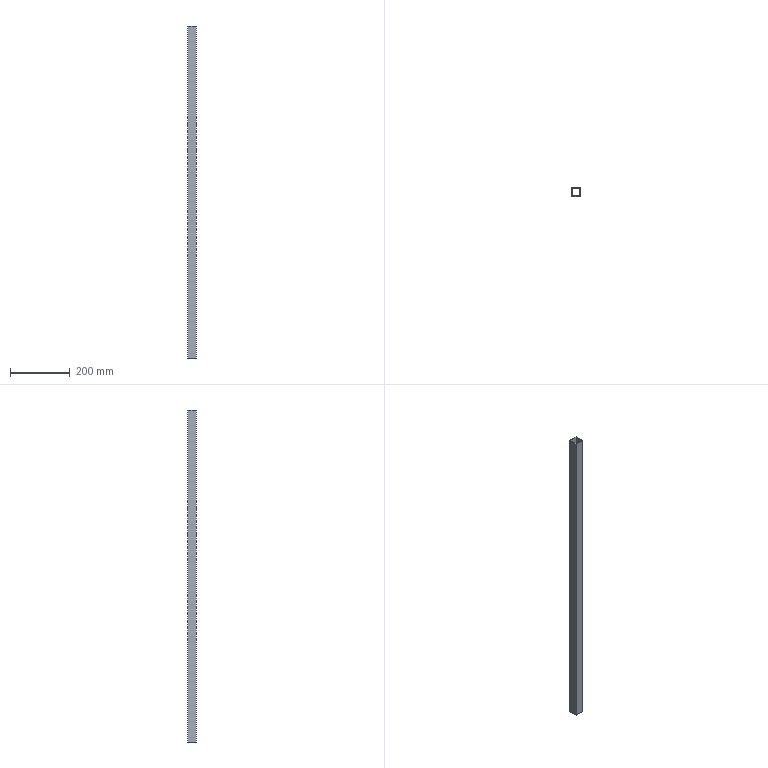Part | SolidWorks | features Extrusion 1 | 1 solid | 10 faces | box 30 x 30 x 1112 mm | volume 249088 mm3 | plane 10
STEP:
#1=CARTESIAN_POINT('',(-15.,15.,556.));
#2=VERTEX_POINT('',#1);
#3=CARTESIAN_POINT('',(-15.,-15.,556.));
#4=VERTEX_POINT('',#3);
#5=CARTESIAN_POINT('',(-15.,-15.,556.));
#6=DIRECTION('',(0.,-1.,0.));
#7=VECTOR('',#6,1000.);
#8=LINE('',#5,#7);
#9=EDGE_CURVE('',#2,#4,#8,.T.);
#10=ORIENTED_EDGE('',*,*,#9,.T.);
#11=CARTESIAN_POINT('',(15.,-15.,556.));
#12=VERTEX_POINT('',#11);
#13=CARTESIAN_POINT('',(15.,-15.,556.));
#14=DIRECTION('',(1.,0.,0.));
#15=VECTOR('',#14,1000.);
#16=LINE('',#13,#15);
#17=EDGE_CURVE('',#4,#12,#16,.T.);
#18=ORIENTED_EDGE('',*,*,#17,.T.);
#19=CARTESIAN_POINT('',(15.,15.,556.));
#20=VERTEX_POINT('',#19);
#21=CARTESIAN_POINT('',(15.,-15.,556.));
#22=DIRECTION('',(0.,1.,0.));
#23=VECTOR('',#22,1000.);
#24=LINE('',#21,#23);
#25=EDGE_CURVE('',#12,#20,#24,.T.);
#26=ORIENTED_EDGE('',*,*,#25,.T.);
#27=CARTESIAN_POINT('',(15.,15.,556.));
#28=DIRECTION('',(-1.,0.,0.));
#29=VECTOR('',#28,1000.);
#30=LINE('',#27,#29);
#31=EDGE_CURVE('',#20,#2,#30,.T.);
#32=ORIENTED_EDGE('',*,*,#31,.T.);
#33=EDGE_LOOP('',(#10,#18,#26,#32));
#34=FACE_OUTER_BOUND('',#33,.T.);
#35=CARTESIAN_POINT('',(13.,13.,556.));
#36=VERTEX_POINT('',#35);
#37=CARTESIAN_POINT('',(-13.,13.,556.));
#38=VERTEX_POINT('',#37);
#39=CARTESIAN_POINT('',(13.,13.,556.));
#40=DIRECTION('',(-1.,0.,0.));
#41=VECTOR('',#40,1000.);
#42=LINE('',#39,#41);
#43=EDGE_CURVE('',#36,#38,#42,.T.);
#44=ORIENTED_EDGE('',*,*,#43,.F.);
#45=CARTESIAN_POINT('',(13.,-13.,556.));
#46=VERTEX_POINT('',#45);
#47=CARTESIAN_POINT('',(13.,-13.,556.));
#48=DIRECTION('',(0.,1.,0.));
#49=VECTOR('',#48,1000.);
#50=LINE('',#47,#49);
#51=EDGE_CURVE('',#46,#36,#50,.T.);
#52=ORIENTED_EDGE('',*,*,#51,.F.);
#53=CARTESIAN_POINT('',(-13.,-13.,556.));
#54=VERTEX_POINT('',#53);
#55=CARTESIAN_POINT('',(13.,-13.,556.));
#56=DIRECTION('',(1.,0.,0.));
#57=VECTOR('',#56,1000.);
#58=LINE('',#55,#57);
#59=EDGE_CURVE('',#54,#46,#58,.T.);
#60=ORIENTED_EDGE('',*,*,#59,.F.);
#61=CARTESIAN_POINT('',(-13.,-13.,556.));
#62=DIRECTION('',(0.,-1.,0.));
#63=VECTOR('',#62,1000.);
#64=LINE('',#61,#63);
#65=EDGE_CURVE('',#38,#54,#64,.T.);
#66=ORIENTED_EDGE('',*,*,#65,.F.);
#67=EDGE_LOOP('',(#44,#52,#60,#66));
#68=FACE_BOUND('',#67,.T.);
#69=CARTESIAN_POINT('',(0.,0.,556.));
#70=DIRECTION('',(0.,0.,1.));
#71=DIRECTION('',(1.,0.,0.));
#72=AXIS2_PLACEMENT_3D('',#69,#70,#71);
#73=PLANE('',#72);
#74=ADVANCED_FACE('',(#34,#68),#73,.T.);
#75=CARTESIAN_POINT('',(-15.,15.,-556.));
#76=VERTEX_POINT('',#75);
#77=CARTESIAN_POINT('',(-15.,-15.,-556.));
#78=VERTEX_POINT('',#77);
#79=CARTESIAN_POINT('',(-15.,-15.,-556.));
#80=DIRECTION('',(0.,-1.,0.));
#81=VECTOR('',#80,1000.);
#82=LINE('',#79,#81);
#83=EDGE_CURVE('',#76,#78,#82,.T.);
#84=ORIENTED_EDGE('',*,*,#83,.F.);
#85=CARTESIAN_POINT('',(15.,15.,-556.));
#86=VERTEX_POINT('',#85);
#87=CARTESIAN_POINT('',(15.,15.,-556.));
#88=DIRECTION('',(-1.,0.,0.));
#89=VECTOR('',#88,1000.);
#90=LINE('',#87,#89);
#91=EDGE_CURVE('',#86,#76,#90,.T.);
#92=ORIENTED_EDGE('',*,*,#91,.F.);
#93=CARTESIAN_POINT('',(15.,-15.,-556.));
#94=VERTEX_POINT('',#93);
#95=CARTESIAN_POINT('',(15.,-15.,-556.));
#96=DIRECTION('',(0.,1.,0.));
#97=VECTOR('',#96,1000.);
#98=LINE('',#95,#97);
#99=EDGE_CURVE('',#94,#86,#98,.T.);
#100=ORIENTED_EDGE('',*,*,#99,.F.);
#101=CARTESIAN_POINT('',(15.,-15.,-556.));
#102=DIRECTION('',(1.,0.,0.));
#103=VECTOR('',#102,1000.);
#104=LINE('',#101,#103);
#105=EDGE_CURVE('',#78,#94,#104,.T.);
#106=ORIENTED_EDGE('',*,*,#105,.F.);
#107=EDGE_LOOP('',(#84,#92,#100,#106));
#108=FACE_OUTER_BOUND('',#107,.T.);
#109=CARTESIAN_POINT('',(13.,-13.,-556.));
#110=VERTEX_POINT('',#109);
#111=CARTESIAN_POINT('',(13.,13.,-556.));
#112=VERTEX_POINT('',#111);
#113=CARTESIAN_POINT('',(13.,-13.,-556.));
#114=DIRECTION('',(0.,1.,0.));
#115=VECTOR('',#114,1000.);
#116=LINE('',#113,#115);
#117=EDGE_CURVE('',#110,#112,#116,.T.);
#118=ORIENTED_EDGE('',*,*,#117,.T.);
#119=CARTESIAN_POINT('',(-13.,13.,-556.));
#120=VERTEX_POINT('',#119);
#121=CARTESIAN_POINT('',(13.,13.,-556.));
#122=DIRECTION('',(-1.,0.,0.));
#123=VECTOR('',#122,1000.);
#124=LINE('',#121,#123);
#125=EDGE_CURVE('',#112,#120,#124,.T.);
#126=ORIENTED_EDGE('',*,*,#125,.T.);
#127=CARTESIAN_POINT('',(-13.,-13.,-556.));
#128=VERTEX_POINT('',#127);
#129=CARTESIAN_POINT('',(-13.,-13.,-556.));
#130=DIRECTION('',(0.,-1.,0.));
#131=VECTOR('',#130,1000.);
#132=LINE('',#129,#131);
#133=EDGE_CURVE('',#120,#128,#132,.T.);
#134=ORIENTED_EDGE('',*,*,#133,.T.);
#135=CARTESIAN_POINT('',(13.,-13.,-556.));
#136=DIRECTION('',(1.,0.,0.));
#137=VECTOR('',#136,1000.);
#138=LINE('',#135,#137);
#139=EDGE_CURVE('',#128,#110,#138,.T.);
#140=ORIENTED_EDGE('',*,*,#139,.T.);
#141=EDGE_LOOP('',(#118,#126,#134,#140));
#142=FACE_BOUND('',#141,.T.);
#143=CARTESIAN_POINT('',(0.,0.,-556.));
#144=DIRECTION('',(0.,0.,1.));
#145=DIRECTION('',(1.,0.,0.));
#146=AXIS2_PLACEMENT_3D('',#143,#144,#145);
#147=PLANE('',#146);
#148=ADVANCED_FACE('',(#108,#142),#147,.F.);
#149=ORIENTED_EDGE('',*,*,#83,.T.);
#150=CARTESIAN_POINT('',(-15.,-15.,556.));
#151=DIRECTION('',(0.,0.,-1.));
#152=VECTOR('',#151,1000.);
#153=LINE('',#150,#152);
#154=EDGE_CURVE('',#4,#78,#153,.T.);
#155=ORIENTED_EDGE('',*,*,#154,.F.);
#156=ORIENTED_EDGE('',*,*,#9,.F.);
#157=CARTESIAN_POINT('',(-15.,15.,556.));
#158=DIRECTION('',(0.,0.,-1.));
#159=VECTOR('',#158,1000.);
#160=LINE('',#157,#159);
#161=EDGE_CURVE('',#2,#76,#160,.T.);
#162=ORIENTED_EDGE('',*,*,#161,.T.);
#163=EDGE_LOOP('',(#149,#155,#156,#162));
#164=FACE_OUTER_BOUND('',#163,.T.);
#165=CARTESIAN_POINT('',(-15.,-15.,556.));
#166=DIRECTION('',(1.,0.,0.));
#167=DIRECTION('',(0.,1.,0.));
#168=AXIS2_PLACEMENT_3D('',#165,#166,#167);
#169=PLANE('',#168);
#170=ADVANCED_FACE('',(#164),#169,.F.);
#171=ORIENTED_EDGE('',*,*,#105,.T.);
#172=CARTESIAN_POINT('',(15.,-15.,556.));
#173=DIRECTION('',(0.,0.,-1.));
#174=VECTOR('',#173,1000.);
#175=LINE('',#172,#174);
#176=EDGE_CURVE('',#12,#94,#175,.T.);
#177=ORIENTED_EDGE('',*,*,#176,.F.);
#178=ORIENTED_EDGE('',*,*,#17,.F.);
#179=ORIENTED_EDGE('',*,*,#154,.T.);
#180=EDGE_LOOP('',(#171,#177,#178,#179));
#181=FACE_OUTER_BOUND('',#180,.T.);
#182=CARTESIAN_POINT('',(15.,-15.,556.));
#183=DIRECTION('',(0.,1.,0.));
#184=DIRECTION('',(-1.,0.,0.));
#185=AXIS2_PLACEMENT_3D('',#182,#183,#184);
#186=PLANE('',#185);
#187=ADVANCED_FACE('',(#181),#186,.F.);
#188=ORIENTED_EDGE('',*,*,#99,.T.);
#189=CARTESIAN_POINT('',(15.,15.,556.));
#190=DIRECTION('',(0.,0.,-1.));
#191=VECTOR('',#190,1000.);
#192=LINE('',#189,#191);
#193=EDGE_CURVE('',#20,#86,#192,.T.);
#194=ORIENTED_EDGE('',*,*,#193,.F.);
#195=ORIENTED_EDGE('',*,*,#25,.F.);
#196=ORIENTED_EDGE('',*,*,#176,.T.);
#197=EDGE_LOOP('',(#188,#194,#195,#196));
#198=FACE_OUTER_BOUND('',#197,.T.);
#199=CARTESIAN_POINT('',(15.,-15.,556.));
#200=DIRECTION('',(-1.,0.,0.));
#201=DIRECTION('',(0.,0.,1.));
#202=AXIS2_PLACEMENT_3D('',#199,#200,#201);
#203=PLANE('',#202);
#204=ADVANCED_FACE('',(#198),#203,.F.);
#205=ORIENTED_EDGE('',*,*,#91,.T.);
#206=ORIENTED_EDGE('',*,*,#161,.F.);
#207=ORIENTED_EDGE('',*,*,#31,.F.);
#208=ORIENTED_EDGE('',*,*,#193,.T.);
#209=EDGE_LOOP('',(#205,#206,#207,#208));
#210=FACE_OUTER_BOUND('',#209,.T.);
#211=CARTESIAN_POINT('',(15.,15.,556.));
#212=DIRECTION('',(0.,-1.,0.));
#213=DIRECTION('',(0.,0.,-1.));
#214=AXIS2_PLACEMENT_3D('',#211,#212,#213);
#215=PLANE('',#214);
#216=ADVANCED_FACE('',(#210),#215,.F.);
#217=ORIENTED_EDGE('',*,*,#117,.F.);
#218=CARTESIAN_POINT('',(13.,-13.,556.));
#219=DIRECTION('',(0.,0.,-1.));
#220=VECTOR('',#219,1000.);
#221=LINE('',#218,#220);
#222=EDGE_CURVE('',#46,#110,#221,.T.);
#223=ORIENTED_EDGE('',*,*,#222,.F.);
#224=ORIENTED_EDGE('',*,*,#51,.T.);
#225=CARTESIAN_POINT('',(13.,13.,556.));
#226=DIRECTION('',(0.,0.,-1.));
#227=VECTOR('',#226,1000.);
#228=LINE('',#225,#227);
#229=EDGE_CURVE('',#36,#112,#228,.T.);
#230=ORIENTED_EDGE('',*,*,#229,.T.);
#231=EDGE_LOOP('',(#217,#223,#224,#230));
#232=FACE_OUTER_BOUND('',#231,.T.);
#233=CARTESIAN_POINT('',(13.,-13.,556.));
#234=DIRECTION('',(-1.,0.,0.));
#235=DIRECTION('',(0.,0.,1.));
#236=AXIS2_PLACEMENT_3D('',#233,#234,#235);
#237=PLANE('',#236);
#238=ADVANCED_FACE('',(#232),#237,.T.);
#239=ORIENTED_EDGE('',*,*,#125,.F.);
#240=ORIENTED_EDGE('',*,*,#229,.F.);
#241=ORIENTED_EDGE('',*,*,#43,.T.);
#242=CARTESIAN_POINT('',(-13.,13.,556.));
#243=DIRECTION('',(0.,0.,-1.));
#244=VECTOR('',#243,1000.);
#245=LINE('',#242,#244);
#246=EDGE_CURVE('',#38,#120,#245,.T.);
#247=ORIENTED_EDGE('',*,*,#246,.T.);
#248=EDGE_LOOP('',(#239,#240,#241,#247));
#249=FACE_OUTER_BOUND('',#248,.T.);
#250=CARTESIAN_POINT('',(13.,13.,556.));
#251=DIRECTION('',(0.,-1.,0.));
#252=DIRECTION('',(0.,0.,-1.));
#253=AXIS2_PLACEMENT_3D('',#250,#251,#252);
#254=PLANE('',#253);
#255=ADVANCED_FACE('',(#249),#254,.T.);
#256=ORIENTED_EDGE('',*,*,#133,.F.);
#257=ORIENTED_EDGE('',*,*,#246,.F.);
#258=ORIENTED_EDGE('',*,*,#65,.T.);
#259=CARTESIAN_POINT('',(-13.,-13.,556.));
#260=DIRECTION('',(0.,0.,-1.));
#261=VECTOR('',#260,1000.);
#262=LINE('',#259,#261);
#263=EDGE_CURVE('',#54,#128,#262,.T.);
#264=ORIENTED_EDGE('',*,*,#263,.T.);
#265=EDGE_LOOP('',(#256,#257,#258,#264));
#266=FACE_OUTER_BOUND('',#265,.T.);
#267=CARTESIAN_POINT('',(-13.,-13.,556.));
#268=DIRECTION('',(1.,0.,0.));
#269=DIRECTION('',(0.,0.,-1.));
#270=AXIS2_PLACEMENT_3D('',#267,#268,#269);
#271=PLANE('',#270);
#272=ADVANCED_FACE('',(#266),#271,.T.);
#273=ORIENTED_EDGE('',*,*,#139,.F.);
#274=ORIENTED_EDGE('',*,*,#263,.F.);
#275=ORIENTED_EDGE('',*,*,#59,.T.);
#276=ORIENTED_EDGE('',*,*,#222,.T.);
#277=EDGE_LOOP('',(#273,#274,#275,#276));
#278=FACE_OUTER_BOUND('',#277,.T.);
#279=CARTESIAN_POINT('',(13.,-13.,556.));
#280=DIRECTION('',(0.,1.,0.));
#281=DIRECTION('',(0.,0.,1.));
#282=AXIS2_PLACEMENT_3D('',#279,#280,#281);
#283=PLANE('',#282);
#284=ADVANCED_FACE('',(#278),#283,.T.);
#285=CLOSED_SHELL('',(#74,#148,#170,#187,#204,#216,#238,#255,#272,#284));
#286=MANIFOLD_SOLID_BREP('',#285);
#287=CARTESIAN_POINT('',(0.,0.,0.));
#288=DIRECTION('',(0.,0.,1.));
#289=DIRECTION('',(1.,0.,0.));
#290=AXIS2_PLACEMENT_3D('',#287,#288,#289);
#291=(LENGTH_UNIT()NAMED_UNIT(*)SI_UNIT(.MILLI.,.METRE.));
#292=UNCERTAINTY_MEASURE_WITH_UNIT(LENGTH_MEASURE(0.00001),#291,'','');
#293=(NAMED_UNIT(*)PLANE_ANGLE_UNIT()SI_UNIT($,.RADIAN.));
#294=(NAMED_UNIT(*)SI_UNIT($,.STERADIAN.)SOLID_ANGLE_UNIT());
#295=(GEOMETRIC_REPRESENTATION_CONTEXT(3)GLOBAL_UNCERTAINTY_ASSIGNED_CONTEXT((#292))GLOBAL_UNIT_ASSIGNED_CONTEXT((#291,#293,#294))REPRESENTATION_CONTEXT('',''));
#296=ADVANCED_BREP_SHAPE_REPRESENTATION('',(#286,#290),#295);